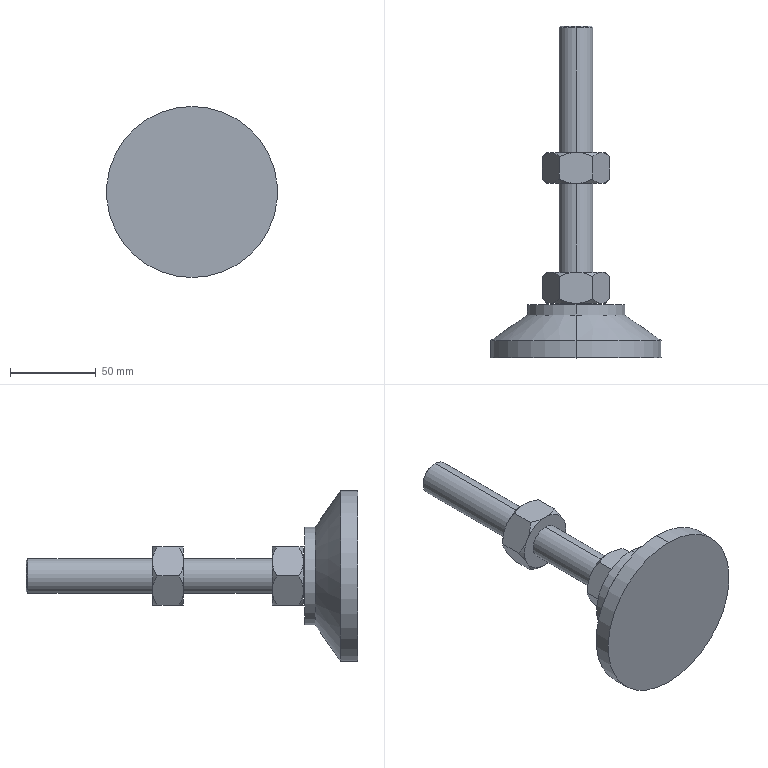Part | SolidWorks | features ICE 2, Chamfer 1, RevCut 1, Revolution 1 | 1 solid | 57 faces | box 100 x 194 x 100 mm | volume 244209 mm3 | cone 28 | plane 19 | cylinder 10 | commonest cylinder face diameters 20 x6 57.156 x2 100 x2